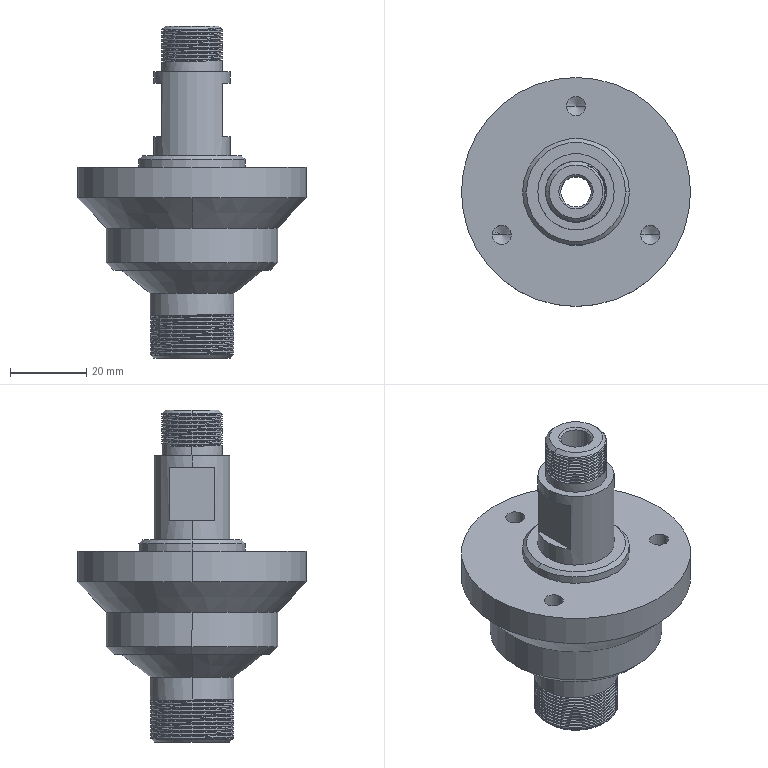Part | NX | features BREP 1 | 1 solid | 100 faces | box 60 x 60 x 87 mm | volume 72276 mm3 | cylinder 58 | cone 24 | plane 14 | spline 4 | commonest cylinder face diameters 22 x22 16 x18 5 x6 8 x2 14 x2 20 x2